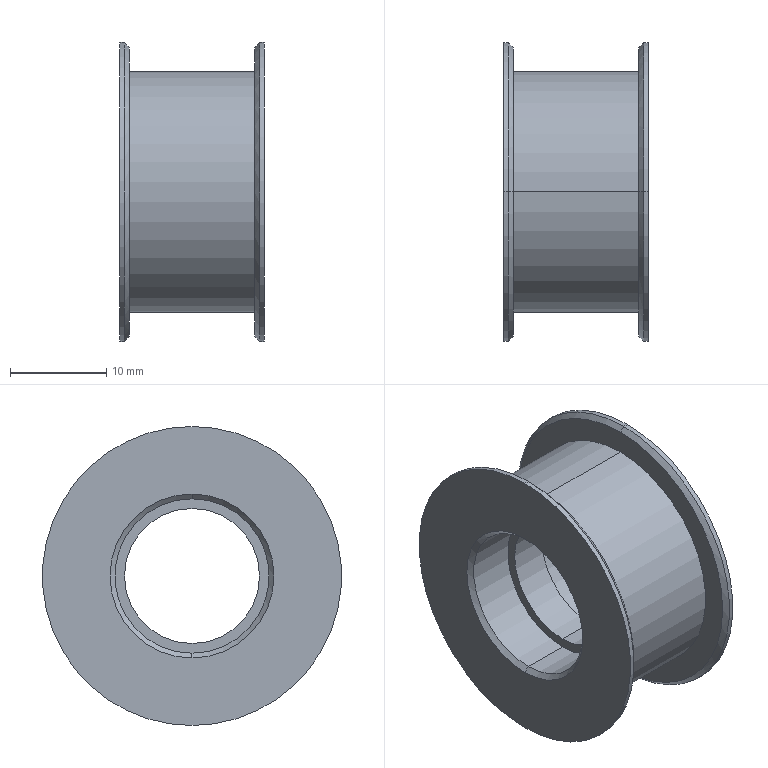Part | NX | features BREP 1 | 1 solid | 26 faces | box 15 x 31 x 31 mm | volume 5027 mm3 | cylinder 12 | cone 8 | plane 6 | commonest cylinder face diameters 16 x4 31 x4 14 x2 25 x2
STEP:
#1=CARTESIAN_POINT('',(6.5,0.,15.));
#2=VERTEX_POINT('',#1);
#3=CARTESIAN_POINT('',(6.5,0.,-15.));
#4=VERTEX_POINT('',#3);
#5=CARTESIAN_POINT('',(6.5,0.,0.));
#6=DIRECTION('',(-1.,0.,0.));
#7=DIRECTION('',(0.,0.,-1.));
#8=AXIS2_PLACEMENT_3D('',#5,#6,#7);
#9=CIRCLE('',#8,15.);
#10=EDGE_CURVE('',#2,#4,#9,.T.);
#11=ORIENTED_EDGE('',*,*,#10,.F.);
#12=CARTESIAN_POINT('',(7.,0.,15.5));
#13=VERTEX_POINT('',#12);
#14=CARTESIAN_POINT('',(6.5,0.,15.));
#15=DIRECTION('',(0.7071,0.,0.7071));
#16=VECTOR('',#15,1000.);
#17=LINE('',#14,#16);
#18=EDGE_CURVE('',#2,#13,#17,.T.);
#19=ORIENTED_EDGE('',*,*,#18,.T.);
#20=CARTESIAN_POINT('',(7.,0.,-15.5));
#21=VERTEX_POINT('',#20);
#22=CARTESIAN_POINT('',(7.,0.,0.));
#23=DIRECTION('',(1.,0.,0.));
#24=DIRECTION('',(0.,0.,-1.));
#25=AXIS2_PLACEMENT_3D('',#22,#23,#24);
#26=CIRCLE('',#25,15.5);
#27=EDGE_CURVE('',#21,#13,#26,.T.);
#28=ORIENTED_EDGE('',*,*,#27,.F.);
#29=CARTESIAN_POINT('',(6.5,0.,-15.));
#30=DIRECTION('',(0.7071,0.,-0.7071));
#31=VECTOR('',#30,1000.);
#32=LINE('',#29,#31);
#33=EDGE_CURVE('',#4,#21,#32,.T.);
#34=ORIENTED_EDGE('',*,*,#33,.F.);
#35=EDGE_LOOP('',(#11,#19,#28,#34));
#36=FACE_BOUND('',#35,.T.);
#37=CARTESIAN_POINT('',(6.5,0.,0.));
#38=DIRECTION('',(1.,0.,0.));
#39=DIRECTION('',(0.,0.,-1.));
#40=AXIS2_PLACEMENT_3D('',#37,#38,#39);
#41=CONICAL_SURFACE('',#40,15.,0.7854);
#42=ADVANCED_FACE('',(#36),#41,.T.);
#43=CARTESIAN_POINT('',(-6.5,0.,-15.));
#44=VERTEX_POINT('',#43);
#45=CARTESIAN_POINT('',(-6.5,0.,15.));
#46=VERTEX_POINT('',#45);
#47=CARTESIAN_POINT('',(-6.5,0.,0.));
#48=DIRECTION('',(1.,0.,0.));
#49=DIRECTION('',(0.,0.,1.));
#50=AXIS2_PLACEMENT_3D('',#47,#48,#49);
#51=CIRCLE('',#50,15.);
#52=EDGE_CURVE('',#44,#46,#51,.T.);
#53=ORIENTED_EDGE('',*,*,#52,.F.);
#54=CARTESIAN_POINT('',(-7.,0.,-15.5));
#55=VERTEX_POINT('',#54);
#56=CARTESIAN_POINT('',(-7.,0.,-15.5));
#57=DIRECTION('',(-0.7071,0.,-0.7071));
#58=VECTOR('',#57,1000.);
#59=LINE('',#56,#58);
#60=EDGE_CURVE('',#55,#44,#59,.F.);
#61=ORIENTED_EDGE('',*,*,#60,.F.);
#62=CARTESIAN_POINT('',(-7.,0.,15.5));
#63=VERTEX_POINT('',#62);
#64=CARTESIAN_POINT('',(-7.,0.,0.));
#65=DIRECTION('',(-1.,0.,0.));
#66=DIRECTION('',(0.,0.,1.));
#67=AXIS2_PLACEMENT_3D('',#64,#65,#66);
#68=CIRCLE('',#67,15.5);
#69=EDGE_CURVE('',#63,#55,#68,.T.);
#70=ORIENTED_EDGE('',*,*,#69,.F.);
#71=CARTESIAN_POINT('',(-7.,0.,15.5));
#72=DIRECTION('',(-0.7071,0.,0.7071));
#73=VECTOR('',#72,1000.);
#74=LINE('',#71,#73);
#75=EDGE_CURVE('',#63,#46,#74,.F.);
#76=ORIENTED_EDGE('',*,*,#75,.T.);
#77=EDGE_LOOP('',(#53,#61,#70,#76));
#78=FACE_BOUND('',#77,.T.);
#79=CARTESIAN_POINT('',(-7.,0.,0.));
#80=DIRECTION('',(-1.,0.,0.));
#81=DIRECTION('',(0.,0.,1.));
#82=AXIS2_PLACEMENT_3D('',#79,#80,#81);
#83=CONICAL_SURFACE('',#82,15.5,0.7854);
#84=ADVANCED_FACE('',(#78),#83,.T.);
#85=CARTESIAN_POINT('',(7.,0.,8.));
#86=VERTEX_POINT('',#85);
#87=CARTESIAN_POINT('',(7.,0.,-8.));
#88=VERTEX_POINT('',#87);
#89=CARTESIAN_POINT('',(7.,0.,0.));
#90=DIRECTION('',(1.,0.,0.));
#91=DIRECTION('',(0.,0.,1.));
#92=AXIS2_PLACEMENT_3D('',#89,#90,#91);
#93=CIRCLE('',#92,8.);
#94=EDGE_CURVE('',#86,#88,#93,.T.);
#95=ORIENTED_EDGE('',*,*,#94,.F.);
#96=CARTESIAN_POINT('',(7.5,0.,8.5));
#97=VERTEX_POINT('',#96);
#98=CARTESIAN_POINT('',(7.5,0.,8.5));
#99=DIRECTION('',(0.7071,0.,0.7071));
#100=VECTOR('',#99,1000.);
#101=LINE('',#98,#100);
#102=EDGE_CURVE('',#86,#97,#101,.T.);
#103=ORIENTED_EDGE('',*,*,#102,.T.);
#104=CARTESIAN_POINT('',(7.5,0.,-8.5));
#105=VERTEX_POINT('',#104);
#106=CARTESIAN_POINT('',(7.5,0.,0.));
#107=DIRECTION('',(-1.,0.,0.));
#108=DIRECTION('',(0.,0.,1.));
#109=AXIS2_PLACEMENT_3D('',#106,#107,#108);
#110=CIRCLE('',#109,8.5);
#111=EDGE_CURVE('',#105,#97,#110,.T.);
#112=ORIENTED_EDGE('',*,*,#111,.F.);
#113=CARTESIAN_POINT('',(7.5,0.,-8.5));
#114=DIRECTION('',(0.7071,0.,-0.7071));
#115=VECTOR('',#114,1000.);
#116=LINE('',#113,#115);
#117=EDGE_CURVE('',#88,#105,#116,.T.);
#118=ORIENTED_EDGE('',*,*,#117,.F.);
#119=EDGE_LOOP('',(#95,#103,#112,#118));
#120=FACE_BOUND('',#119,.T.);
#121=CARTESIAN_POINT('',(7.5,0.,0.));
#122=DIRECTION('',(1.,0.,0.));
#123=DIRECTION('',(0.,0.,-1.));
#124=AXIS2_PLACEMENT_3D('',#121,#122,#123);
#125=CONICAL_SURFACE('',#124,8.5,0.7854);
#126=ADVANCED_FACE('',(#120),#125,.F.);
#127=CARTESIAN_POINT('',(-7.,0.,-8.));
#128=VERTEX_POINT('',#127);
#129=CARTESIAN_POINT('',(-7.,0.,8.));
#130=VERTEX_POINT('',#129);
#131=CARTESIAN_POINT('',(-7.,0.,0.));
#132=DIRECTION('',(-1.,0.,0.));
#133=DIRECTION('',(0.,0.,-1.));
#134=AXIS2_PLACEMENT_3D('',#131,#132,#133);
#135=CIRCLE('',#134,8.);
#136=EDGE_CURVE('',#128,#130,#135,.T.);
#137=ORIENTED_EDGE('',*,*,#136,.F.);
#138=CARTESIAN_POINT('',(-7.5,0.,-8.5));
#139=VERTEX_POINT('',#138);
#140=CARTESIAN_POINT('',(-7.,0.,-8.));
#141=DIRECTION('',(-0.7071,0.,-0.7071));
#142=VECTOR('',#141,1000.);
#143=LINE('',#140,#142);
#144=EDGE_CURVE('',#139,#128,#143,.F.);
#145=ORIENTED_EDGE('',*,*,#144,.F.);
#146=CARTESIAN_POINT('',(-7.5,0.,8.5));
#147=VERTEX_POINT('',#146);
#148=CARTESIAN_POINT('',(-7.5,0.,0.));
#149=DIRECTION('',(1.,0.,0.));
#150=DIRECTION('',(0.,0.,-1.));
#151=AXIS2_PLACEMENT_3D('',#148,#149,#150);
#152=CIRCLE('',#151,8.5);
#153=EDGE_CURVE('',#147,#139,#152,.T.);
#154=ORIENTED_EDGE('',*,*,#153,.F.);
#155=CARTESIAN_POINT('',(-7.,0.,8.));
#156=DIRECTION('',(-0.7071,0.,0.7071));
#157=VECTOR('',#156,1000.);
#158=LINE('',#155,#157);
#159=EDGE_CURVE('',#147,#130,#158,.F.);
#160=ORIENTED_EDGE('',*,*,#159,.T.);
#161=EDGE_LOOP('',(#137,#145,#154,#160));
#162=FACE_BOUND('',#161,.T.);
#163=CARTESIAN_POINT('',(-7.,0.,0.));
#164=DIRECTION('',(-1.,0.,0.));
#165=DIRECTION('',(0.,0.,1.));
#166=AXIS2_PLACEMENT_3D('',#163,#164,#165);
#167=CONICAL_SURFACE('',#166,8.,0.7854);
#168=ADVANCED_FACE('',(#162),#167,.F.);
#169=CARTESIAN_POINT('',(2.,0.,7.));
#170=VERTEX_POINT('',#169);
#171=CARTESIAN_POINT('',(2.,0.,-7.));
#172=VERTEX_POINT('',#171);
#173=CARTESIAN_POINT('',(2.,0.,0.));
#174=DIRECTION('',(1.,0.,0.));
#175=DIRECTION('',(0.,0.,-1.));
#176=AXIS2_PLACEMENT_3D('',#173,#174,#175);
#177=CIRCLE('',#176,7.);
#178=EDGE_CURVE('',#170,#172,#177,.T.);
#179=ORIENTED_EDGE('',*,*,#178,.T.);
#180=CARTESIAN_POINT('',(-2.,0.,-7.));
#181=VERTEX_POINT('',#180);
#182=CARTESIAN_POINT('',(2.,0.,-7.));
#183=DIRECTION('',(-1.,0.,0.));
#184=VECTOR('',#183,1000.);
#185=LINE('',#182,#184);
#186=EDGE_CURVE('',#181,#172,#185,.F.);
#187=ORIENTED_EDGE('',*,*,#186,.F.);
#188=CARTESIAN_POINT('',(-2.,0.,7.));
#189=VERTEX_POINT('',#188);
#190=CARTESIAN_POINT('',(-2.,0.,0.));
#191=DIRECTION('',(1.,0.,0.));
#192=DIRECTION('',(0.,0.,-1.));
#193=AXIS2_PLACEMENT_3D('',#190,#191,#192);
#194=CIRCLE('',#193,7.);
#195=EDGE_CURVE('',#189,#181,#194,.T.);
#196=ORIENTED_EDGE('',*,*,#195,.F.);
#197=CARTESIAN_POINT('',(2.,0.,7.));
#198=DIRECTION('',(-1.,0.,0.));
#199=VECTOR('',#198,1000.);
#200=LINE('',#197,#199);
#201=EDGE_CURVE('',#189,#170,#200,.F.);
#202=ORIENTED_EDGE('',*,*,#201,.T.);
#203=EDGE_LOOP('',(#179,#187,#196,#202));
#204=FACE_BOUND('',#203,.T.);
#205=CARTESIAN_POINT('',(2.,0.,0.));
#206=DIRECTION('',(-1.,0.,0.));
#207=DIRECTION('',(0.,0.,1.));
#208=AXIS2_PLACEMENT_3D('',#205,#206,#207);
#209=CYLINDRICAL_SURFACE('',#208,7.);
#210=ADVANCED_FACE('',(#204),#209,.F.);
#211=ORIENTED_EDGE('',*,*,#69,.T.);
#212=CARTESIAN_POINT('',(-7.5,0.,-15.5));
#213=VERTEX_POINT('',#212);
#214=CARTESIAN_POINT('',(0.,0.,-15.5));
#215=DIRECTION('',(-1.,0.,0.));
#216=VECTOR('',#215,1000.);
#217=LINE('',#214,#216);
#218=EDGE_CURVE('',#213,#55,#217,.F.);
#219=ORIENTED_EDGE('',*,*,#218,.F.);
#220=CARTESIAN_POINT('',(-7.5,0.,15.5));
#221=VERTEX_POINT('',#220);
#222=CARTESIAN_POINT('',(-7.5,0.,0.));
#223=DIRECTION('',(-1.,0.,0.));
#224=DIRECTION('',(0.,0.,1.));
#225=AXIS2_PLACEMENT_3D('',#222,#223,#224);
#226=CIRCLE('',#225,15.5);
#227=EDGE_CURVE('',#221,#213,#226,.T.);
#228=ORIENTED_EDGE('',*,*,#227,.F.);
#229=CARTESIAN_POINT('',(0.,0.,15.5));
#230=DIRECTION('',(-1.,0.,0.));
#231=VECTOR('',#230,1000.);
#232=LINE('',#229,#231);
#233=EDGE_CURVE('',#221,#63,#232,.F.);
#234=ORIENTED_EDGE('',*,*,#233,.T.);
#235=EDGE_LOOP('',(#211,#219,#228,#234));
#236=FACE_BOUND('',#235,.T.);
#237=CARTESIAN_POINT('',(0.,0.,0.));
#238=DIRECTION('',(-1.,0.,0.));
#239=DIRECTION('',(0.,0.,1.));
#240=AXIS2_PLACEMENT_3D('',#237,#238,#239);
#241=CYLINDRICAL_SURFACE('',#240,15.5);
#242=ADVANCED_FACE('',(#236),#241,.T.);
#243=CARTESIAN_POINT('',(6.5,0.,12.5));
#244=VERTEX_POINT('',#243);
#245=CARTESIAN_POINT('',(6.5,0.,-12.5));
#246=VERTEX_POINT('',#245);
#247=CARTESIAN_POINT('',(6.5,0.,0.));
#248=DIRECTION('',(-1.,0.,0.));
#249=DIRECTION('',(0.,0.,1.));
#250=AXIS2_PLACEMENT_3D('',#247,#248,#249);
#251=CIRCLE('',#250,12.5);
#252=EDGE_CURVE('',#244,#246,#251,.T.);
#253=ORIENTED_EDGE('',*,*,#252,.T.);
#254=CARTESIAN_POINT('',(-6.5,0.,-12.5));
#255=VERTEX_POINT('',#254);
#256=CARTESIAN_POINT('',(0.,0.,-12.5));
#257=DIRECTION('',(-1.,0.,0.));
#258=VECTOR('',#257,1000.);
#259=LINE('',#256,#258);
#260=EDGE_CURVE('',#255,#246,#259,.F.);
#261=ORIENTED_EDGE('',*,*,#260,.F.);
#262=CARTESIAN_POINT('',(-6.5,0.,12.5));
#263=VERTEX_POINT('',#262);
#264=CARTESIAN_POINT('',(-6.5,0.,0.));
#265=DIRECTION('',(-1.,0.,0.));
#266=DIRECTION('',(0.,0.,1.));
#267=AXIS2_PLACEMENT_3D('',#264,#265,#266);
#268=CIRCLE('',#267,12.5);
#269=EDGE_CURVE('',#263,#255,#268,.T.);
#270=ORIENTED_EDGE('',*,*,#269,.F.);
#271=CARTESIAN_POINT('',(0.,0.,12.5));
#272=DIRECTION('',(-1.,0.,0.));
#273=VECTOR('',#272,1000.);
#274=LINE('',#271,#273);
#275=EDGE_CURVE('',#263,#244,#274,.F.);
#276=ORIENTED_EDGE('',*,*,#275,.T.);
#277=EDGE_LOOP('',(#253,#261,#270,#276));
#278=FACE_BOUND('',#277,.T.);
#279=CARTESIAN_POINT('',(0.,0.,0.));
#280=DIRECTION('',(-1.,0.,0.));
#281=DIRECTION('',(0.,0.,1.));
#282=AXIS2_PLACEMENT_3D('',#279,#280,#281);
#283=CYLINDRICAL_SURFACE('',#282,12.5);
#284=ADVANCED_FACE('',(#278),#283,.T.);
#285=CARTESIAN_POINT('',(7.5,0.,15.5));
#286=VERTEX_POINT('',#285);
#287=CARTESIAN_POINT('',(7.5,0.,-15.5));
#288=VERTEX_POINT('',#287);
#289=CARTESIAN_POINT('',(7.5,0.,0.));
#290=DIRECTION('',(-1.,0.,0.));
#291=DIRECTION('',(0.,0.,1.));
#292=AXIS2_PLACEMENT_3D('',#289,#290,#291);
#293=CIRCLE('',#292,15.5);
#294=EDGE_CURVE('',#286,#288,#293,.T.);
#295=ORIENTED_EDGE('',*,*,#294,.T.);
#296=CARTESIAN_POINT('',(0.,0.,-15.5));
#297=DIRECTION('',(-1.,0.,0.));
#298=VECTOR('',#297,1000.);
#299=LINE('',#296,#298);
#300=EDGE_CURVE('',#21,#288,#299,.F.);
#301=ORIENTED_EDGE('',*,*,#300,.F.);
#302=ORIENTED_EDGE('',*,*,#27,.T.);
#303=CARTESIAN_POINT('',(0.,0.,15.5));
#304=DIRECTION('',(-1.,0.,0.));
#305=VECTOR('',#304,1000.);
#306=LINE('',#303,#305);
#307=EDGE_CURVE('',#13,#286,#306,.F.);
#308=ORIENTED_EDGE('',*,*,#307,.T.);
#309=EDGE_LOOP('',(#295,#301,#302,#308));
#310=FACE_BOUND('',#309,.T.);
#311=CARTESIAN_POINT('',(0.,0.,0.));
#312=DIRECTION('',(-1.,0.,0.));
#313=DIRECTION('',(0.,0.,1.));
#314=AXIS2_PLACEMENT_3D('',#311,#312,#313);
#315=CYLINDRICAL_SURFACE('',#314,15.5);
#316=ADVANCED_FACE('',(#310),#315,.T.);
#317=ORIENTED_EDGE('',*,*,#94,.T.);
#318=CARTESIAN_POINT('',(2.,0.,-8.));
#319=VERTEX_POINT('',#318);
#320=CARTESIAN_POINT('',(0.,0.,-8.));
#321=DIRECTION('',(-1.,0.,0.));
#322=VECTOR('',#321,1000.);
#323=LINE('',#320,#322);
#324=EDGE_CURVE('',#319,#88,#323,.F.);
#325=ORIENTED_EDGE('',*,*,#324,.F.);
#326=CARTESIAN_POINT('',(2.,0.,8.));
#327=VERTEX_POINT('',#326);
#328=CARTESIAN_POINT('',(2.,0.,0.));
#329=DIRECTION('',(1.,0.,0.));
#330=DIRECTION('',(0.,0.,-1.));
#331=AXIS2_PLACEMENT_3D('',#328,#329,#330);
#332=CIRCLE('',#331,8.);
#333=EDGE_CURVE('',#327,#319,#332,.T.);
#334=ORIENTED_EDGE('',*,*,#333,.F.);
#335=CARTESIAN_POINT('',(0.,0.,8.));
#336=DIRECTION('',(-1.,0.,0.));
#337=VECTOR('',#336,1000.);
#338=LINE('',#335,#337);
#339=EDGE_CURVE('',#327,#86,#338,.F.);
#340=ORIENTED_EDGE('',*,*,#339,.T.);
#341=EDGE_LOOP('',(#317,#325,#334,#340));
#342=FACE_BOUND('',#341,.T.);
#343=CARTESIAN_POINT('',(0.,0.,0.));
#344=DIRECTION('',(-1.,0.,0.));
#345=DIRECTION('',(0.,0.,1.));
#346=AXIS2_PLACEMENT_3D('',#343,#344,#345);
#347=CYLINDRICAL_SURFACE('',#346,8.);
#348=ADVANCED_FACE('',(#342),#347,.F.);
#349=CARTESIAN_POINT('',(-2.,0.,-8.));
#350=VERTEX_POINT('',#349);
#351=CARTESIAN_POINT('',(-2.,0.,8.));
#352=VERTEX_POINT('',#351);
#353=CARTESIAN_POINT('',(-2.,0.,0.));
#354=DIRECTION('',(-1.,0.,0.));
#355=DIRECTION('',(0.,0.,-1.));
#356=AXIS2_PLACEMENT_3D('',#353,#354,#355);
#357=CIRCLE('',#356,8.);
#358=EDGE_CURVE('',#350,#352,#357,.T.);
#359=ORIENTED_EDGE('',*,*,#358,.F.);
#360=CARTESIAN_POINT('',(0.,0.,-8.));
#361=DIRECTION('',(-1.,0.,0.));
#362=VECTOR('',#361,1000.);
#363=LINE('',#360,#362);
#364=EDGE_CURVE('',#128,#350,#363,.F.);
#365=ORIENTED_EDGE('',*,*,#364,.F.);
#366=ORIENTED_EDGE('',*,*,#136,.T.);
#367=CARTESIAN_POINT('',(0.,0.,8.));
#368=DIRECTION('',(-1.,0.,0.));
#369=VECTOR('',#368,1000.);
#370=LINE('',#367,#369);
#371=EDGE_CURVE('',#130,#352,#370,.F.);
#372=ORIENTED_EDGE('',*,*,#371,.T.);
#373=EDGE_LOOP('',(#359,#365,#366,#372));
#374=FACE_BOUND('',#373,.T.);
#375=CARTESIAN_POINT('',(0.,0.,0.));
#376=DIRECTION('',(-1.,0.,0.));
#377=DIRECTION('',(0.,0.,1.));
#378=AXIS2_PLACEMENT_3D('',#375,#376,#377);
#379=CYLINDRICAL_SURFACE('',#378,8.);
#380=ADVANCED_FACE('',(#374),#379,.F.);
#381=ORIENTED_EDGE('',*,*,#364,.T.);
#382=CARTESIAN_POINT('',(-2.,0.,0.));
#383=DIRECTION('',(-1.,0.,0.));
#384=DIRECTION('',(0.,0.,-1.));
#385=AXIS2_PLACEMENT_3D('',#382,#383,#384);
#386=CIRCLE('',#385,8.);
#387=EDGE_CURVE('',#352,#350,#386,.T.);
#388=ORIENTED_EDGE('',*,*,#387,.F.);
#389=ORIENTED_EDGE('',*,*,#371,.F.);
#390=CARTESIAN_POINT('',(-7.,0.,0.));
#391=DIRECTION('',(-1.,0.,0.));
#392=DIRECTION('',(0.,0.,-1.));
#393=AXIS2_PLACEMENT_3D('',#390,#391,#392);
#394=CIRCLE('',#393,8.);
#395=EDGE_CURVE('',#130,#128,#394,.T.);
#396=ORIENTED_EDGE('',*,*,#395,.T.);
#397=EDGE_LOOP('',(#381,#388,#389,#396));
#398=FACE_BOUND('',#397,.T.);
#399=CARTESIAN_POINT('',(0.,0.,0.));
#400=DIRECTION('',(-1.,0.,0.));
#401=DIRECTION('',(0.,0.,1.));
#402=AXIS2_PLACEMENT_3D('',#399,#400,#401);
#403=CYLINDRICAL_SURFACE('',#402,8.);
#404=ADVANCED_FACE('',(#398),#403,.F.);
#405=ORIENTED_EDGE('',*,*,#227,.T.);
#406=CARTESIAN_POINT('',(-7.5,0.,0.));
#407=DIRECTION('',(-1.,0.,0.));
#408=DIRECTION('',(0.,0.,1.));
#409=AXIS2_PLACEMENT_3D('',#406,#407,#408);
#410=CIRCLE('',#409,15.5);
#411=EDGE_CURVE('',#213,#221,#410,.T.);
#412=ORIENTED_EDGE('',*,*,#411,.T.);
#413=EDGE_LOOP('',(#405,#412));
#414=FACE_BOUND('',#413,.T.);
#415=ORIENTED_EDGE('',*,*,#153,.T.);
#416=CARTESIAN_POINT('',(-7.5,0.,0.));
#417=DIRECTION('',(1.,0.,0.));
#418=DIRECTION('',(0.,0.,-1.));
#419=AXIS2_PLACEMENT_3D('',#416,#417,#418);
#420=CIRCLE('',#419,8.5);
#421=EDGE_CURVE('',#139,#147,#420,.T.);
#422=ORIENTED_EDGE('',*,*,#421,.T.);
#423=EDGE_LOOP('',(#415,#422));
#424=FACE_BOUND('',#423,.T.);
#425=CARTESIAN_POINT('',(-7.5,15.5,0.));
#426=DIRECTION('',(1.,0.,0.));
#427=DIRECTION('',(0.,1.,0.));
#428=AXIS2_PLACEMENT_3D('',#425,#426,#427);
#429=PLANE('',#428);
#430=ADVANCED_FACE('',(#414,#424),#429,.F.);
#431=ORIENTED_EDGE('',*,*,#324,.T.);
#432=CARTESIAN_POINT('',(7.,0.,0.));
#433=DIRECTION('',(1.,0.,0.));
#434=DIRECTION('',(0.,0.,1.));
#435=AXIS2_PLACEMENT_3D('',#432,#433,#434);
#436=CIRCLE('',#435,8.);
#437=EDGE_CURVE('',#88,#86,#436,.T.);
#438=ORIENTED_EDGE('',*,*,#437,.T.);
#439=ORIENTED_EDGE('',*,*,#339,.F.);
#440=CARTESIAN_POINT('',(2.,0.,0.));
#441=DIRECTION('',(1.,0.,0.));
#442=DIRECTION('',(0.,0.,-1.));
#443=AXIS2_PLACEMENT_3D('',#440,#441,#442);
#444=CIRCLE('',#443,8.);
#445=EDGE_CURVE('',#319,#327,#444,.T.);
#446=ORIENTED_EDGE('',*,*,#445,.F.);
#447=EDGE_LOOP('',(#431,#438,#439,#446));
#448=FACE_BOUND('',#447,.T.);
#449=CARTESIAN_POINT('',(0.,0.,0.));
#450=DIRECTION('',(-1.,0.,0.));
#451=DIRECTION('',(0.,0.,1.));
#452=AXIS2_PLACEMENT_3D('',#449,#450,#451);
#453=CYLINDRICAL_SURFACE('',#452,8.);
#454=ADVANCED_FACE('',(#448),#453,.F.);
#455=ORIENTED_EDGE('',*,*,#294,.F.);
#456=CARTESIAN_POINT('',(7.5,0.,0.));
#457=DIRECTION('',(-1.,0.,0.));
#458=DIRECTION('',(0.,0.,1.));
#459=AXIS2_PLACEMENT_3D('',#456,#457,#458);
#460=CIRCLE('',#459,15.5);
#461=EDGE_CURVE('',#288,#286,#460,.T.);
#462=ORIENTED_EDGE('',*,*,#461,.F.);
#463=EDGE_LOOP('',(#455,#462));
#464=FACE_BOUND('',#463,.T.);
#465=ORIENTED_EDGE('',*,*,#111,.T.);
#466=CARTESIAN_POINT('',(7.5,0.,0.));
#467=DIRECTION('',(-1.,0.,0.));
#468=DIRECTION('',(0.,0.,1.));
#469=AXIS2_PLACEMENT_3D('',#466,#467,#468);
#470=CIRCLE('',#469,8.5);
#471=EDGE_CURVE('',#97,#105,#470,.T.);
#472=ORIENTED_EDGE('',*,*,#471,.T.);
#473=EDGE_LOOP('',(#465,#472));
#474=FACE_BOUND('',#473,.T.);
#475=CARTESIAN_POINT('',(7.5,15.5,0.));
#476=DIRECTION('',(-1.,0.,0.));
#477=DIRECTION('',(0.,0.,1.));
#478=AXIS2_PLACEMENT_3D('',#475,#476,#477);
#479=PLANE('',#478);
#480=ADVANCED_FACE('',(#464,#474),#479,.F.);
#481=ORIENTED_EDGE('',*,*,#300,.T.);
#482=ORIENTED_EDGE('',*,*,#461,.T.);
#483=ORIENTED_EDGE('',*,*,#307,.F.);
#484=CARTESIAN_POINT('',(7.,0.,0.));
#485=DIRECTION('',(1.,0.,0.));
#486=DIRECTION('',(0.,0.,-1.));
#487=AXIS2_PLACEMENT_3D('',#484,#485,#486);
#488=CIRCLE('',#487,15.5);
#489=EDGE_CURVE('',#13,#21,#488,.T.);
#490=ORIENTED_EDGE('',*,*,#489,.T.);
#491=EDGE_LOOP('',(#481,#482,#483,#490));
#492=FACE_BOUND('',#491,.T.);
#493=CARTESIAN_POINT('',(0.,0.,0.));
#494=DIRECTION('',(-1.,0.,0.));
#495=DIRECTION('',(0.,0.,1.));
#496=AXIS2_PLACEMENT_3D('',#493,#494,#495);
#497=CYLINDRICAL_SURFACE('',#496,15.5);
#498=ADVANCED_FACE('',(#492),#497,.T.);
#499=CARTESIAN_POINT('',(6.5,0.,0.));
#500=DIRECTION('',(-1.,0.,0.));
#501=DIRECTION('',(0.,0.,-1.));
#502=AXIS2_PLACEMENT_3D('',#499,#500,#501);
#503=CIRCLE('',#502,15.);
#504=EDGE_CURVE('',#4,#2,#503,.T.);
#505=ORIENTED_EDGE('',*,*,#504,.T.);
#506=ORIENTED_EDGE('',*,*,#10,.T.);
#507=EDGE_LOOP('',(#505,#506));
#508=FACE_BOUND('',#507,.T.);
#509=ORIENTED_EDGE('',*,*,#252,.F.);
#510=CARTESIAN_POINT('',(6.5,0.,0.));
#511=DIRECTION('',(-1.,0.,0.));
#512=DIRECTION('',(0.,0.,1.));
#513=AXIS2_PLACEMENT_3D('',#510,#511,#512);
#514=CIRCLE('',#513,12.5);
#515=EDGE_CURVE('',#246,#244,#514,.T.);
#516=ORIENTED_EDGE('',*,*,#515,.F.);
#517=EDGE_LOOP('',(#509,#516));
#518=FACE_BOUND('',#517,.T.);
#519=CARTESIAN_POINT('',(6.5,15.5,0.));
#520=DIRECTION('',(1.,0.,0.));
#521=DIRECTION('',(0.,1.,0.));
#522=AXIS2_PLACEMENT_3D('',#519,#520,#521);
#523=PLANE('',#522);
#524=ADVANCED_FACE('',(#508,#518),#523,.F.);
#525=ORIENTED_EDGE('',*,*,#260,.T.);
#526=ORIENTED_EDGE('',*,*,#515,.T.);
#527=ORIENTED_EDGE('',*,*,#275,.F.);
#528=CARTESIAN_POINT('',(-6.5,0.,0.));
#529=DIRECTION('',(-1.,0.,0.));
#530=DIRECTION('',(0.,0.,1.));
#531=AXIS2_PLACEMENT_3D('',#528,#529,#530);
#532=CIRCLE('',#531,12.5);
#533=EDGE_CURVE('',#255,#263,#532,.T.);
#534=ORIENTED_EDGE('',*,*,#533,.F.);
#535=EDGE_LOOP('',(#525,#526,#527,#534));
#536=FACE_BOUND('',#535,.T.);
#537=CARTESIAN_POINT('',(0.,0.,0.));
#538=DIRECTION('',(-1.,0.,0.));
#539=DIRECTION('',(0.,0.,1.));
#540=AXIS2_PLACEMENT_3D('',#537,#538,#539);
#541=CYLINDRICAL_SURFACE('',#540,12.5);
#542=ADVANCED_FACE('',(#536),#541,.T.);
#543=CARTESIAN_POINT('',(-6.5,0.,0.));
#544=DIRECTION('',(1.,0.,0.));
#545=DIRECTION('',(0.,0.,1.));
#546=AXIS2_PLACEMENT_3D('',#543,#544,#545);
#547=CIRCLE('',#546,15.);
#548=EDGE_CURVE('',#46,#44,#547,.T.);
#549=ORIENTED_EDGE('',*,*,#548,.T.);
#550=ORIENTED_EDGE('',*,*,#52,.T.);
#551=EDGE_LOOP('',(#549,#550));
#552=FACE_BOUND('',#551,.T.);
#553=ORIENTED_EDGE('',*,*,#269,.T.);
#554=ORIENTED_EDGE('',*,*,#533,.T.);
#555=EDGE_LOOP('',(#553,#554));
#556=FACE_BOUND('',#555,.T.);
#557=CARTESIAN_POINT('',(-6.5,15.5,0.));
#558=DIRECTION('',(-1.,0.,0.));
#559=DIRECTION('',(0.,0.,1.));
#560=AXIS2_PLACEMENT_3D('',#557,#558,#559);
#561=PLANE('',#560);
#562=ADVANCED_FACE('',(#552,#556),#561,.F.);
#563=ORIENTED_EDGE('',*,*,#218,.T.);
#564=CARTESIAN_POINT('',(-7.,0.,0.));
#565=DIRECTION('',(-1.,0.,0.));
#566=DIRECTION('',(0.,0.,1.));
#567=AXIS2_PLACEMENT_3D('',#564,#565,#566);
#568=CIRCLE('',#567,15.5);
#569=EDGE_CURVE('',#55,#63,#568,.T.);
#570=ORIENTED_EDGE('',*,*,#569,.T.);
#571=ORIENTED_EDGE('',*,*,#233,.F.);
#572=ORIENTED_EDGE('',*,*,#411,.F.);
#573=EDGE_LOOP('',(#563,#570,#571,#572));
#574=FACE_BOUND('',#573,.T.);
#575=CARTESIAN_POINT('',(0.,0.,0.));
#576=DIRECTION('',(-1.,0.,0.));
#577=DIRECTION('',(0.,0.,1.));
#578=AXIS2_PLACEMENT_3D('',#575,#576,#577);
#579=CYLINDRICAL_SURFACE('',#578,15.5);
#580=ADVANCED_FACE('',(#574),#579,.T.);
#581=ORIENTED_EDGE('',*,*,#333,.T.);
#582=ORIENTED_EDGE('',*,*,#445,.T.);
#583=EDGE_LOOP('',(#581,#582));
#584=FACE_BOUND('',#583,.T.);
#585=ORIENTED_EDGE('',*,*,#178,.F.);
#586=CARTESIAN_POINT('',(2.,0.,0.));
#587=DIRECTION('',(1.,0.,0.));
#588=DIRECTION('',(0.,0.,-1.));
#589=AXIS2_PLACEMENT_3D('',#586,#587,#588);
#590=CIRCLE('',#589,7.);
#591=EDGE_CURVE('',#172,#170,#590,.T.);
#592=ORIENTED_EDGE('',*,*,#591,.F.);
#593=EDGE_LOOP('',(#585,#592));
#594=FACE_BOUND('',#593,.T.);
#595=CARTESIAN_POINT('',(2.,0.,0.));
#596=DIRECTION('',(1.,0.,0.));
#597=DIRECTION('',(0.,1.,0.));
#598=AXIS2_PLACEMENT_3D('',#595,#596,#597);
#599=PLANE('',#598);
#600=ADVANCED_FACE('',(#584,#594),#599,.T.);
#601=ORIENTED_EDGE('',*,*,#387,.T.);
#602=ORIENTED_EDGE('',*,*,#358,.T.);
#603=EDGE_LOOP('',(#601,#602));
#604=FACE_BOUND('',#603,.T.);
#605=ORIENTED_EDGE('',*,*,#195,.T.);
#606=CARTESIAN_POINT('',(-2.,0.,0.));
#607=DIRECTION('',(1.,0.,0.));
#608=DIRECTION('',(0.,0.,-1.));
#609=AXIS2_PLACEMENT_3D('',#606,#607,#608);
#610=CIRCLE('',#609,7.);
#611=EDGE_CURVE('',#181,#189,#610,.T.);
#612=ORIENTED_EDGE('',*,*,#611,.T.);
#613=EDGE_LOOP('',(#605,#612));
#614=FACE_BOUND('',#613,.T.);
#615=CARTESIAN_POINT('',(-2.,0.,0.));
#616=DIRECTION('',(1.,0.,0.));
#617=DIRECTION('',(0.,1.,0.));
#618=AXIS2_PLACEMENT_3D('',#615,#616,#617);
#619=PLANE('',#618);
#620=ADVANCED_FACE('',(#604,#614),#619,.F.);
#621=ORIENTED_EDGE('',*,*,#186,.T.);
#622=ORIENTED_EDGE('',*,*,#591,.T.);
#623=ORIENTED_EDGE('',*,*,#201,.F.);
#624=ORIENTED_EDGE('',*,*,#611,.F.);
#625=EDGE_LOOP('',(#621,#622,#623,#624));
#626=FACE_BOUND('',#625,.T.);
#627=CARTESIAN_POINT('',(2.,0.,0.));
#628=DIRECTION('',(-1.,0.,0.));
#629=DIRECTION('',(0.,0.,1.));
#630=AXIS2_PLACEMENT_3D('',#627,#628,#629);
#631=CYLINDRICAL_SURFACE('',#630,7.);
#632=ADVANCED_FACE('',(#626),#631,.F.);
#633=ORIENTED_EDGE('',*,*,#144,.T.);
#634=ORIENTED_EDGE('',*,*,#395,.F.);
#635=ORIENTED_EDGE('',*,*,#159,.F.);
#636=ORIENTED_EDGE('',*,*,#421,.F.);
#637=EDGE_LOOP('',(#633,#634,#635,#636));
#638=FACE_BOUND('',#637,.T.);
#639=CARTESIAN_POINT('',(-7.,0.,0.));
#640=DIRECTION('',(-1.,0.,0.));
#641=DIRECTION('',(0.,0.,1.));
#642=AXIS2_PLACEMENT_3D('',#639,#640,#641);
#643=CONICAL_SURFACE('',#642,8.,0.7854);
#644=ADVANCED_FACE('',(#638),#643,.F.);
#645=ORIENTED_EDGE('',*,*,#102,.F.);
#646=ORIENTED_EDGE('',*,*,#437,.F.);
#647=ORIENTED_EDGE('',*,*,#117,.T.);
#648=ORIENTED_EDGE('',*,*,#471,.F.);
#649=EDGE_LOOP('',(#645,#646,#647,#648));
#650=FACE_BOUND('',#649,.T.);
#651=CARTESIAN_POINT('',(7.5,0.,0.));
#652=DIRECTION('',(1.,0.,0.));
#653=DIRECTION('',(0.,0.,-1.));
#654=AXIS2_PLACEMENT_3D('',#651,#652,#653);
#655=CONICAL_SURFACE('',#654,8.5,0.7854);
#656=ADVANCED_FACE('',(#650),#655,.F.);
#657=ORIENTED_EDGE('',*,*,#60,.T.);
#658=ORIENTED_EDGE('',*,*,#548,.F.);
#659=ORIENTED_EDGE('',*,*,#75,.F.);
#660=ORIENTED_EDGE('',*,*,#569,.F.);
#661=EDGE_LOOP('',(#657,#658,#659,#660));
#662=FACE_BOUND('',#661,.T.);
#663=CARTESIAN_POINT('',(-7.,0.,0.));
#664=DIRECTION('',(-1.,0.,0.));
#665=DIRECTION('',(0.,0.,1.));
#666=AXIS2_PLACEMENT_3D('',#663,#664,#665);
#667=CONICAL_SURFACE('',#666,15.5,0.7854);
#668=ADVANCED_FACE('',(#662),#667,.T.);
#669=ORIENTED_EDGE('',*,*,#18,.F.);
#670=ORIENTED_EDGE('',*,*,#504,.F.);
#671=ORIENTED_EDGE('',*,*,#33,.T.);
#672=ORIENTED_EDGE('',*,*,#489,.F.);
#673=EDGE_LOOP('',(#669,#670,#671,#672));
#674=FACE_BOUND('',#673,.T.);
#675=CARTESIAN_POINT('',(6.5,0.,0.));
#676=DIRECTION('',(1.,0.,0.));
#677=DIRECTION('',(0.,0.,-1.));
#678=AXIS2_PLACEMENT_3D('',#675,#676,#677);
#679=CONICAL_SURFACE('',#678,15.,0.7854);
#680=ADVANCED_FACE('',(#674),#679,.T.);
#681=CLOSED_SHELL('',(#42,#84,#126,#168,#210,#242,#284,#316,#348,#380,#404,#430,#454,#480,#498,#524,#542,#562,#580,#600,#620,#632,#644,#656,#668,#680));
#682=MANIFOLD_SOLID_BREP('',#681);
#683=(LENGTH_UNIT()NAMED_UNIT(*)SI_UNIT(.MILLI.,.METRE.));
#684=UNCERTAINTY_MEASURE_WITH_UNIT(LENGTH_MEASURE(0.00001),#683,'','');
#685=(NAMED_UNIT(*)PLANE_ANGLE_UNIT()SI_UNIT($,.RADIAN.));
#686=(NAMED_UNIT(*)SI_UNIT($,.STERADIAN.)SOLID_ANGLE_UNIT());
#687=(GEOMETRIC_REPRESENTATION_CONTEXT(3)GLOBAL_UNCERTAINTY_ASSIGNED_CONTEXT((#684))GLOBAL_UNIT_ASSIGNED_CONTEXT((#683,#685,#686))REPRESENTATION_CONTEXT('',''));
#688=ADVANCED_BREP_SHAPE_REPRESENTATION('',(#682),#687);